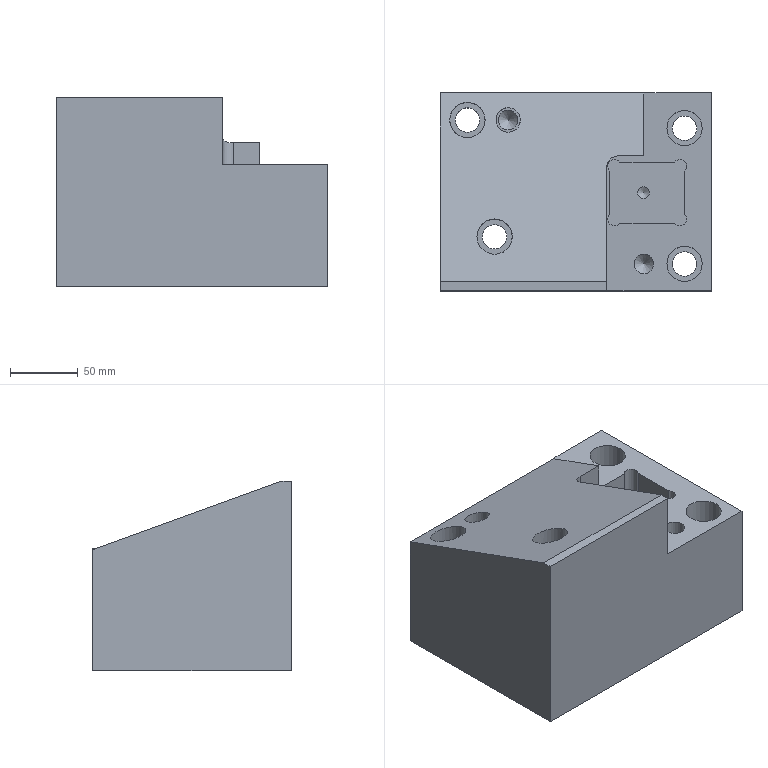Part | STEP file | lll_id5022_x_t | 1 solid | 42 faces | box 200 x 146 x 140 mm | volume 2863405 mm3 | plane 22 | cylinder 17 | cone 3 | commonest cylinder face diameters 10 x4 18.009 x4 26.008 x4 14.506 x2 8.506 x1 16 x1
STEP:
#1=CARTESIAN_POINT('',(2866.996,-53.,0.));
#2=VERTEX_POINT('',#1);
#3=CARTESIAN_POINT('',(2880.,-53.,0.));
#4=DIRECTION('',(0.,0.,1.));
#5=DIRECTION('',(-1.,0.,0.));
#6=AXIS2_PLACEMENT_3D('',#3,#4,#5);
#7=CIRCLE('',#6,13.004);
#8=EDGE_CURVE('',#2,#2,#7,.T.);
#9=ORIENTED_EDGE('',*,*,#8,.F.);
#10=EDGE_LOOP('',(#9));
#11=FACE_BOUND('',#10,.T.);
#12=CARTESIAN_POINT('',(2866.996,-153.,0.));
#13=VERTEX_POINT('',#12);
#14=CARTESIAN_POINT('',(2880.,-153.,0.));
#15=DIRECTION('',(0.,0.,1.));
#16=DIRECTION('',(-1.,0.,0.));
#17=AXIS2_PLACEMENT_3D('',#14,#15,#16);
#18=CIRCLE('',#17,13.004);
#19=EDGE_CURVE('',#13,#13,#18,.T.);
#20=ORIENTED_EDGE('',*,*,#19,.F.);
#21=EDGE_LOOP('',(#20));
#22=FACE_BOUND('',#21,.T.);
#23=CARTESIAN_POINT('',(2822.75,-173.,0.));
#24=VERTEX_POINT('',#23);
#25=CARTESIAN_POINT('',(2822.75,-81.5,0.));
#26=VERTEX_POINT('',#25);
#27=CARTESIAN_POINT('',(2822.75,-150.5,0.));
#28=DIRECTION('',(0.,1.,0.));
#29=VECTOR('',#28,1.);
#30=LINE('',#27,#29);
#31=EDGE_CURVE('',#24,#26,#30,.T.);
#32=ORIENTED_EDGE('',*,*,#31,.F.);
#33=CARTESIAN_POINT('',(2900.,-173.,0.));
#34=VERTEX_POINT('',#33);
#35=CARTESIAN_POINT('',(2692.5,-173.,0.));
#36=DIRECTION('',(-1.,0.,0.));
#37=VECTOR('',#36,1.);
#38=LINE('',#35,#37);
#39=EDGE_CURVE('',#34,#24,#38,.T.);
#40=ORIENTED_EDGE('',*,*,#39,.F.);
#41=CARTESIAN_POINT('',(2900.,-27.,0.));
#42=VERTEX_POINT('',#41);
#43=CARTESIAN_POINT('',(2900.,0.00007613,0.));
#44=DIRECTION('',(0.,1.,0.));
#45=VECTOR('',#44,1.);
#46=LINE('',#43,#45);
#47=EDGE_CURVE('',#34,#42,#46,.T.);
#48=ORIENTED_EDGE('',*,*,#47,.T.);
#49=CARTESIAN_POINT('',(2850.,-27.,0.));
#50=VERTEX_POINT('',#49);
#51=CARTESIAN_POINT('',(2520.,-27.,0.));
#52=DIRECTION('',(1.,0.,0.));
#53=VECTOR('',#52,1.);
#54=LINE('',#51,#53);
#55=EDGE_CURVE('',#50,#42,#54,.T.);
#56=ORIENTED_EDGE('',*,*,#55,.F.);
#57=CARTESIAN_POINT('',(2850.,-28.941,0.));
#58=VERTEX_POINT('',#57);
#59=CARTESIAN_POINT('',(2850.,-102.5,0.));
#60=DIRECTION('',(0.,1.,0.));
#61=VECTOR('',#60,1.);
#62=LINE('',#59,#61);
#63=EDGE_CURVE('',#58,#50,#62,.T.);
#64=ORIENTED_EDGE('',*,*,#63,.F.);
#65=CARTESIAN_POINT('',(2850.,-73.5,0.));
#66=VERTEX_POINT('',#65);
#67=CARTESIAN_POINT('',(2850.,-97.5,0.));
#68=DIRECTION('',(0.,-1.,0.));
#69=VECTOR('',#68,1.);
#70=LINE('',#67,#69);
#71=EDGE_CURVE('',#58,#66,#70,.T.);
#72=ORIENTED_EDGE('',*,*,#71,.T.);
#73=CARTESIAN_POINT('',(2830.75,-73.5,0.));
#74=VERTEX_POINT('',#73);
#75=CARTESIAN_POINT('',(2839.75,-73.5,0.));
#76=DIRECTION('',(1.,0.,0.));
#77=VECTOR('',#76,1.);
#78=LINE('',#75,#77);
#79=EDGE_CURVE('',#74,#66,#78,.T.);
#80=ORIENTED_EDGE('',*,*,#79,.F.);
#81=CARTESIAN_POINT('',(2830.75,-81.5,0.));
#82=DIRECTION('',(0.,0.,-1.));
#83=DIRECTION('',(-1.,0.,0.));
#84=AXIS2_PLACEMENT_3D('',#81,#82,#83);
#85=CIRCLE('',#84,8.);
#86=EDGE_CURVE('',#26,#74,#85,.T.);
#87=ORIENTED_EDGE('',*,*,#86,.F.);
#88=EDGE_LOOP('',(#32,#40,#48,#56,#64,#72,#80,#87));
#89=FACE_BOUND('',#88,.T.);
#90=CARTESIAN_POINT('',(2879.963,-116.273,0.));
#91=VERTEX_POINT('',#90);
#92=CARTESIAN_POINT('',(2879.963,-84.727,0.));
#93=VERTEX_POINT('',#92);
#94=CARTESIAN_POINT('',(2879.963,0.00007613,0.));
#95=DIRECTION('',(0.,1.,0.));
#96=VECTOR('',#95,1.);
#97=LINE('',#94,#96);
#98=EDGE_CURVE('',#91,#93,#97,.T.);
#99=ORIENTED_EDGE('',*,*,#98,.F.);
#100=CARTESIAN_POINT('',(2872.626,-123.,0.));
#101=VERTEX_POINT('',#100);
#102=CARTESIAN_POINT('',(2876.618,-119.989,0.));
#103=DIRECTION('',(0.,0.,1.));
#104=DIRECTION('',(-1.,0.,0.));
#105=AXIS2_PLACEMENT_3D('',#102,#103,#104);
#106=CIRCLE('',#105,5.);
#107=EDGE_CURVE('',#101,#91,#106,.T.);
#108=ORIENTED_EDGE('',*,*,#107,.F.);
#109=CARTESIAN_POINT('',(2832.3,-123.,0.));
#110=VERTEX_POINT('',#109);
#111=CARTESIAN_POINT('',(2772.5,-123.,0.));
#112=DIRECTION('',(1.,0.,0.));
#113=VECTOR('',#112,1.);
#114=LINE('',#111,#113);
#115=EDGE_CURVE('',#110,#101,#114,.T.);
#116=ORIENTED_EDGE('',*,*,#115,.F.);
#117=CARTESIAN_POINT('',(2824.963,-116.273,0.));
#118=VERTEX_POINT('',#117);
#119=CARTESIAN_POINT('',(2828.308,-119.989,0.));
#120=DIRECTION('',(0.,0.,1.));
#121=DIRECTION('',(-1.,0.,0.));
#122=AXIS2_PLACEMENT_3D('',#119,#120,#121);
#123=CIRCLE('',#122,5.);
#124=EDGE_CURVE('',#118,#110,#123,.T.);
#125=ORIENTED_EDGE('',*,*,#124,.F.);
#126=CARTESIAN_POINT('',(2824.963,-84.727,0.));
#127=VERTEX_POINT('',#126);
#128=CARTESIAN_POINT('',(2824.963,0.00007613,0.));
#129=DIRECTION('',(0.,-1.,0.));
#130=VECTOR('',#129,1.);
#131=LINE('',#128,#130);
#132=EDGE_CURVE('',#127,#118,#131,.T.);
#133=ORIENTED_EDGE('',*,*,#132,.F.);
#134=CARTESIAN_POINT('',(2832.3,-78.,0.));
#135=VERTEX_POINT('',#134);
#136=CARTESIAN_POINT('',(2828.308,-81.01,0.));
#137=DIRECTION('',(0.,0.,1.));
#138=DIRECTION('',(-1.,0.,0.));
#139=AXIS2_PLACEMENT_3D('',#136,#137,#138);
#140=CIRCLE('',#139,5.);
#141=EDGE_CURVE('',#135,#127,#140,.T.);
#142=ORIENTED_EDGE('',*,*,#141,.F.);
#143=CARTESIAN_POINT('',(2872.626,-78.,0.));
#144=VERTEX_POINT('',#143);
#145=CARTESIAN_POINT('',(2772.5,-78.,0.));
#146=DIRECTION('',(-1.,0.,0.));
#147=VECTOR('',#146,1.);
#148=LINE('',#145,#147);
#149=EDGE_CURVE('',#144,#135,#148,.T.);
#150=ORIENTED_EDGE('',*,*,#149,.F.);
#151=CARTESIAN_POINT('',(2876.618,-81.01,0.));
#152=DIRECTION('',(0.,0.,1.));
#153=DIRECTION('',(-1.,0.,0.));
#154=AXIS2_PLACEMENT_3D('',#151,#152,#153);
#155=CIRCLE('',#154,5.);
#156=EDGE_CURVE('',#93,#144,#155,.T.);
#157=ORIENTED_EDGE('',*,*,#156,.F.);
#158=EDGE_LOOP('',(#99,#108,#116,#125,#133,#142,#150,#157));
#159=FACE_BOUND('',#158,.T.);
#160=CARTESIAN_POINT('',(2842.747,-153.,0.));
#161=VERTEX_POINT('',#160);
#162=CARTESIAN_POINT('',(2850.,-153.,0.));
#163=DIRECTION('',(0.,0.,-1.));
#164=DIRECTION('',(-1.,0.,0.));
#165=AXIS2_PLACEMENT_3D('',#162,#163,#164);
#166=CIRCLE('',#165,7.253);
#167=EDGE_CURVE('',#161,#161,#166,.T.);
#168=ORIENTED_EDGE('',*,*,#167,.T.);
#169=EDGE_LOOP('',(#168));
#170=FACE_BOUND('',#169,.T.);
#171=CARTESIAN_POINT('',(2772.5,0.00007613,0.));
#172=DIRECTION('',(0.,0.,1.));
#173=DIRECTION('',(1.,0.,0.));
#174=AXIS2_PLACEMENT_3D('',#171,#172,#173);
#175=PLANE('',#174);
#176=ADVANCED_FACE('',(#11,#22,#89,#159,#170),#175,.T.);
#177=CARTESIAN_POINT('',(2822.75,-173.,50.));
#178=VERTEX_POINT('',#177);
#179=CARTESIAN_POINT('',(2700.,-173.,50.));
#180=VERTEX_POINT('',#179);
#181=CARTESIAN_POINT('',(2692.5,-173.,50.));
#182=DIRECTION('',(-1.,0.,0.));
#183=VECTOR('',#182,1.);
#184=LINE('',#181,#183);
#185=EDGE_CURVE('',#178,#180,#184,.T.);
#186=ORIENTED_EDGE('',*,*,#185,.T.);
#187=CARTESIAN_POINT('',(2700.,-173.,-90.));
#188=VERTEX_POINT('',#187);
#189=CARTESIAN_POINT('',(2700.,-173.,6.));
#190=DIRECTION('',(0.,0.,-1.));
#191=VECTOR('',#190,1.);
#192=LINE('',#189,#191);
#193=EDGE_CURVE('',#180,#188,#192,.T.);
#194=ORIENTED_EDGE('',*,*,#193,.T.);
#195=CARTESIAN_POINT('',(2900.,-173.,-90.));
#196=VERTEX_POINT('',#195);
#197=CARTESIAN_POINT('',(-2196.249,-173.,-90.));
#198=DIRECTION('',(1.,0.,0.));
#199=VECTOR('',#198,1.);
#200=LINE('',#197,#199);
#201=EDGE_CURVE('',#188,#196,#200,.T.);
#202=ORIENTED_EDGE('',*,*,#201,.T.);
#203=CARTESIAN_POINT('',(2900.,-173.,-80.));
#204=DIRECTION('',(0.,0.,1.));
#205=VECTOR('',#204,1.);
#206=LINE('',#203,#205);
#207=EDGE_CURVE('',#196,#34,#206,.T.);
#208=ORIENTED_EDGE('',*,*,#207,.T.);
#209=ORIENTED_EDGE('',*,*,#39,.T.);
#210=CARTESIAN_POINT('',(2822.75,-173.,6.));
#211=DIRECTION('',(0.,0.,1.));
#212=VECTOR('',#211,1.);
#213=LINE('',#210,#212);
#214=EDGE_CURVE('',#24,#178,#213,.T.);
#215=ORIENTED_EDGE('',*,*,#214,.T.);
#216=EDGE_LOOP('',(#186,#194,#202,#208,#209,#215));
#217=FACE_OUTER_BOUND('',#216,.T.);
#218=CARTESIAN_POINT('',(2692.5,-173.,6.));
#219=DIRECTION('',(0.,-1.,0.));
#220=DIRECTION('',(0.,0.,-1.));
#221=AXIS2_PLACEMENT_3D('',#218,#219,#220);
#222=PLANE('',#221);
#223=ADVANCED_FACE('',(#217),#222,.T.);
#224=CARTESIAN_POINT('',(2700.,-27.,-90.));
#225=VERTEX_POINT('',#224);
#226=CARTESIAN_POINT('',(2700.,-27.,-0.7065));
#227=VERTEX_POINT('',#226);
#228=CARTESIAN_POINT('',(2700.,-27.,-80.));
#229=DIRECTION('',(0.,0.,1.));
#230=VECTOR('',#229,1.);
#231=LINE('',#228,#230);
#232=EDGE_CURVE('',#225,#227,#231,.T.);
#233=ORIENTED_EDGE('',*,*,#232,.T.);
#234=CARTESIAN_POINT('',(2850.,-27.,-0.7065));
#235=VERTEX_POINT('',#234);
#236=CARTESIAN_POINT('',(2872.426,-27.,-0.7065));
#237=DIRECTION('',(1.,0.,0.));
#238=VECTOR('',#237,1.);
#239=LINE('',#236,#238);
#240=EDGE_CURVE('',#227,#235,#239,.T.);
#241=ORIENTED_EDGE('',*,*,#240,.T.);
#242=CARTESIAN_POINT('',(2850.,-27.,-80.));
#243=DIRECTION('',(0.,0.,1.));
#244=VECTOR('',#243,1.);
#245=LINE('',#242,#244);
#246=EDGE_CURVE('',#235,#50,#245,.T.);
#247=ORIENTED_EDGE('',*,*,#246,.T.);
#248=ORIENTED_EDGE('',*,*,#55,.T.);
#249=CARTESIAN_POINT('',(2900.,-27.,-90.));
#250=VERTEX_POINT('',#249);
#251=CARTESIAN_POINT('',(2900.,-27.,-80.));
#252=DIRECTION('',(0.,0.,1.));
#253=VECTOR('',#252,1.);
#254=LINE('',#251,#253);
#255=EDGE_CURVE('',#250,#42,#254,.T.);
#256=ORIENTED_EDGE('',*,*,#255,.F.);
#257=CARTESIAN_POINT('',(-2196.249,-27.,-90.));
#258=DIRECTION('',(1.,0.,0.));
#259=VECTOR('',#258,1.);
#260=LINE('',#257,#259);
#261=EDGE_CURVE('',#225,#250,#260,.T.);
#262=ORIENTED_EDGE('',*,*,#261,.F.);
#263=EDGE_LOOP('',(#233,#241,#247,#248,#256,#262));
#264=FACE_OUTER_BOUND('',#263,.T.);
#265=CARTESIAN_POINT('',(2520.,-27.,-80.));
#266=DIRECTION('',(0.,-1.,0.));
#267=DIRECTION('',(0.,0.,1.));
#268=AXIS2_PLACEMENT_3D('',#265,#266,#267);
#269=PLANE('',#268);
#270=ADVANCED_FACE('',(#264),#269,.F.);
#271=CARTESIAN_POINT('',(2740.,-119.996,33.141));
#272=VERTEX_POINT('',#271);
#273=CARTESIAN_POINT('',(2740.,-133.,37.874));
#274=DIRECTION('',(0.,-0.342,-0.9397));
#275=DIRECTION('',(0.,0.9397,-0.342));
#276=AXIS2_PLACEMENT_3D('',#273,#274,#275);
#277=ELLIPSE('',#276,13.839,13.004);
#278=EDGE_CURVE('',#272,#272,#277,.T.);
#279=ORIENTED_EDGE('',*,*,#278,.T.);
#280=EDGE_LOOP('',(#279));
#281=FACE_BOUND('',#280,.T.);
#282=CARTESIAN_POINT('',(2720.,-33.996,1.84));
#283=VERTEX_POINT('',#282);
#284=CARTESIAN_POINT('',(2720.,-47.,6.573));
#285=DIRECTION('',(0.,-0.342,-0.9397));
#286=DIRECTION('',(0.,0.9397,-0.342));
#287=AXIS2_PLACEMENT_3D('',#284,#285,#286);
#288=ELLIPSE('',#287,13.839,13.004);
#289=EDGE_CURVE('',#283,#283,#288,.T.);
#290=ORIENTED_EDGE('',*,*,#289,.T.);
#291=EDGE_LOOP('',(#290));
#292=FACE_BOUND('',#291,.T.);
#293=CARTESIAN_POINT('',(2750.,-38.,3.297));
#294=VERTEX_POINT('',#293);
#295=CARTESIAN_POINT('',(2750.,-47.,6.573));
#296=DIRECTION('',(0.,-0.342,-0.9397));
#297=DIRECTION('',(0.,0.9397,-0.342));
#298=AXIS2_PLACEMENT_3D('',#295,#296,#297);
#299=ELLIPSE('',#298,9.578,9.);
#300=EDGE_CURVE('',#294,#294,#299,.T.);
#301=ORIENTED_EDGE('',*,*,#300,.T.);
#302=EDGE_LOOP('',(#301));
#303=FACE_BOUND('',#302,.T.);
#304=CARTESIAN_POINT('',(2700.,-166.315,50.));
#305=VERTEX_POINT('',#304);
#306=CARTESIAN_POINT('',(2822.75,-166.315,50.));
#307=VERTEX_POINT('',#306);
#308=CARTESIAN_POINT('',(2872.426,-166.315,50.));
#309=DIRECTION('',(1.,0.,0.));
#310=VECTOR('',#309,1.);
#311=LINE('',#308,#310);
#312=EDGE_CURVE('',#305,#307,#311,.T.);
#313=ORIENTED_EDGE('',*,*,#312,.T.);
#314=CARTESIAN_POINT('',(2822.75,-81.5,19.13));
#315=VERTEX_POINT('',#314);
#316=CARTESIAN_POINT('',(2822.75,-20.898,-2.927));
#317=DIRECTION('',(0.,0.9397,-0.342));
#318=VECTOR('',#317,1.);
#319=LINE('',#316,#318);
#320=EDGE_CURVE('',#307,#315,#319,.T.);
#321=ORIENTED_EDGE('',*,*,#320,.T.);
#322=CARTESIAN_POINT('',(2830.75,-73.5,16.218));
#323=VERTEX_POINT('',#322);
#324=CARTESIAN_POINT('',(2830.75,-81.5,19.13));
#325=DIRECTION('',(0.,0.342,0.9397));
#326=DIRECTION('',(0.,-0.9397,0.342));
#327=AXIS2_PLACEMENT_3D('',#324,#325,#326);
#328=ELLIPSE('',#327,8.513,8.);
#329=EDGE_CURVE('',#323,#315,#328,.T.);
#330=ORIENTED_EDGE('',*,*,#329,.F.);
#331=CARTESIAN_POINT('',(2850.,-73.5,16.218));
#332=VERTEX_POINT('',#331);
#333=CARTESIAN_POINT('',(2872.426,-73.5,16.218));
#334=DIRECTION('',(1.,0.,0.));
#335=VECTOR('',#334,1.);
#336=LINE('',#333,#335);
#337=EDGE_CURVE('',#323,#332,#336,.T.);
#338=ORIENTED_EDGE('',*,*,#337,.T.);
#339=CARTESIAN_POINT('',(2850.,-20.898,-2.927));
#340=DIRECTION('',(0.,-0.9397,0.342));
#341=VECTOR('',#340,1.);
#342=LINE('',#339,#341);
#343=EDGE_CURVE('',#58,#332,#342,.T.);
#344=ORIENTED_EDGE('',*,*,#343,.F.);
#345=CARTESIAN_POINT('',(2850.,-85.693,20.656));
#346=DIRECTION('',(0.,-0.9397,0.342));
#347=VECTOR('',#346,1.);
#348=LINE('',#345,#347);
#349=EDGE_CURVE('',#235,#58,#348,.T.);
#350=ORIENTED_EDGE('',*,*,#349,.F.);
#351=ORIENTED_EDGE('',*,*,#240,.F.);
#352=CARTESIAN_POINT('',(2700.,-20.898,-2.927));
#353=DIRECTION('',(0.,0.9397,-0.342));
#354=VECTOR('',#353,1.);
#355=LINE('',#352,#354);
#356=EDGE_CURVE('',#305,#227,#355,.T.);
#357=ORIENTED_EDGE('',*,*,#356,.F.);
#358=EDGE_LOOP('',(#313,#321,#330,#338,#344,#350,#351,#357));
#359=FACE_BOUND('',#358,.T.);
#360=CARTESIAN_POINT('',(2872.426,-20.898,-2.927));
#361=DIRECTION('',(0.,0.342,0.9397));
#362=DIRECTION('',(0.,-0.9397,0.342));
#363=AXIS2_PLACEMENT_3D('',#360,#361,#362);
#364=PLANE('',#363);
#365=ADVANCED_FACE('',(#281,#292,#303,#359),#364,.T.);
#366=CARTESIAN_POINT('',(2749.004,-133.,-90.));
#367=VERTEX_POINT('',#366);
#368=CARTESIAN_POINT('',(2740.,-133.,-90.));
#369=DIRECTION('',(0.,0.,1.));
#370=DIRECTION('',(1.,0.,0.));
#371=AXIS2_PLACEMENT_3D('',#368,#369,#370);
#372=CIRCLE('',#371,9.005);
#373=EDGE_CURVE('',#367,#367,#372,.T.);
#374=ORIENTED_EDGE('',*,*,#373,.T.);
#375=EDGE_LOOP('',(#374));
#376=FACE_BOUND('',#375,.T.);
#377=CARTESIAN_POINT('',(2729.004,-47.,-90.));
#378=VERTEX_POINT('',#377);
#379=CARTESIAN_POINT('',(2720.,-47.,-90.));
#380=DIRECTION('',(0.,0.,1.));
#381=DIRECTION('',(1.,0.,0.));
#382=AXIS2_PLACEMENT_3D('',#379,#380,#381);
#383=CIRCLE('',#382,9.005);
#384=EDGE_CURVE('',#378,#378,#383,.T.);
#385=ORIENTED_EDGE('',*,*,#384,.T.);
#386=EDGE_LOOP('',(#385));
#387=FACE_BOUND('',#386,.T.);
#388=CARTESIAN_POINT('',(2889.005,-53.,-90.));
#389=VERTEX_POINT('',#388);
#390=CARTESIAN_POINT('',(2880.,-53.,-90.));
#391=DIRECTION('',(0.,0.,1.));
#392=DIRECTION('',(1.,0.,0.));
#393=AXIS2_PLACEMENT_3D('',#390,#391,#392);
#394=CIRCLE('',#393,9.005);
#395=EDGE_CURVE('',#389,#389,#394,.T.);
#396=ORIENTED_EDGE('',*,*,#395,.T.);
#397=EDGE_LOOP('',(#396));
#398=FACE_BOUND('',#397,.T.);
#399=CARTESIAN_POINT('',(2889.005,-153.,-90.));
#400=VERTEX_POINT('',#399);
#401=CARTESIAN_POINT('',(2880.,-153.,-90.));
#402=DIRECTION('',(0.,0.,1.));
#403=DIRECTION('',(1.,0.,0.));
#404=AXIS2_PLACEMENT_3D('',#401,#402,#403);
#405=CIRCLE('',#404,9.005);
#406=EDGE_CURVE('',#400,#400,#405,.T.);
#407=ORIENTED_EDGE('',*,*,#406,.T.);
#408=EDGE_LOOP('',(#407));
#409=FACE_BOUND('',#408,.T.);
#410=ORIENTED_EDGE('',*,*,#261,.T.);
#411=CARTESIAN_POINT('',(2900.,1.,-90.));
#412=DIRECTION('',(0.,1.,0.));
#413=VECTOR('',#412,1.);
#414=LINE('',#411,#413);
#415=EDGE_CURVE('',#196,#250,#414,.T.);
#416=ORIENTED_EDGE('',*,*,#415,.F.);
#417=ORIENTED_EDGE('',*,*,#201,.F.);
#418=CARTESIAN_POINT('',(2700.,-97.5,-90.));
#419=DIRECTION('',(0.,1.,0.));
#420=VECTOR('',#419,1.);
#421=LINE('',#418,#420);
#422=EDGE_CURVE('',#188,#225,#421,.T.);
#423=ORIENTED_EDGE('',*,*,#422,.T.);
#424=EDGE_LOOP('',(#410,#416,#417,#423));
#425=FACE_BOUND('',#424,.T.);
#426=CARTESIAN_POINT('',(-2196.249,1.,-90.));
#427=DIRECTION('',(0.,0.,-1.));
#428=DIRECTION('',(1.,0.,0.));
#429=AXIS2_PLACEMENT_3D('',#426,#427,#428);
#430=PLANE('',#429);
#431=ADVANCED_FACE('',(#376,#387,#398,#409,#425),#430,.T.);
#432=ORIENTED_EDGE('',*,*,#79,.T.);
#433=CARTESIAN_POINT('',(2850.,-73.5,0.));
#434=DIRECTION('',(0.,0.,1.));
#435=VECTOR('',#434,1.);
#436=LINE('',#433,#435);
#437=EDGE_CURVE('',#66,#332,#436,.T.);
#438=ORIENTED_EDGE('',*,*,#437,.T.);
#439=ORIENTED_EDGE('',*,*,#337,.F.);
#440=CARTESIAN_POINT('',(2830.75,-73.5,16.218));
#441=DIRECTION('',(0.,0.,1.));
#442=VECTOR('',#441,1.);
#443=LINE('',#440,#442);
#444=EDGE_CURVE('',#74,#323,#443,.T.);
#445=ORIENTED_EDGE('',*,*,#444,.F.);
#446=EDGE_LOOP('',(#432,#438,#439,#445));
#447=FACE_OUTER_BOUND('',#446,.T.);
#448=CARTESIAN_POINT('',(2839.75,-73.5,0.));
#449=DIRECTION('',(0.,1.,0.));
#450=DIRECTION('',(0.,0.,1.));
#451=AXIS2_PLACEMENT_3D('',#448,#449,#450);
#452=PLANE('',#451);
#453=ADVANCED_FACE('',(#447),#452,.F.);
#454=ORIENTED_EDGE('',*,*,#214,.F.);
#455=ORIENTED_EDGE('',*,*,#31,.T.);
#456=CARTESIAN_POINT('',(2822.75,-81.5,0.));
#457=DIRECTION('',(0.,0.,-1.));
#458=VECTOR('',#457,1.);
#459=LINE('',#456,#458);
#460=EDGE_CURVE('',#315,#26,#459,.T.);
#461=ORIENTED_EDGE('',*,*,#460,.F.);
#462=ORIENTED_EDGE('',*,*,#320,.F.);
#463=CARTESIAN_POINT('',(2822.75,97.5,50.));
#464=DIRECTION('',(0.,-1.,0.));
#465=VECTOR('',#464,1.);
#466=LINE('',#463,#465);
#467=EDGE_CURVE('',#307,#178,#466,.T.);
#468=ORIENTED_EDGE('',*,*,#467,.T.);
#469=EDGE_LOOP('',(#454,#455,#461,#462,#468));
#470=FACE_OUTER_BOUND('',#469,.T.);
#471=CARTESIAN_POINT('',(2822.75,-150.5,0.));
#472=DIRECTION('',(-1.,0.,0.));
#473=DIRECTION('',(0.,0.,-1.));
#474=AXIS2_PLACEMENT_3D('',#471,#472,#473);
#475=PLANE('',#474);
#476=ADVANCED_FACE('',(#470),#475,.F.);
#477=ORIENTED_EDGE('',*,*,#71,.F.);
#478=ORIENTED_EDGE('',*,*,#343,.T.);
#479=ORIENTED_EDGE('',*,*,#437,.F.);
#480=EDGE_LOOP('',(#477,#478,#479));
#481=FACE_OUTER_BOUND('',#480,.T.);
#482=CARTESIAN_POINT('',(2850.,-97.5,-25.521));
#483=DIRECTION('',(1.,0.,0.));
#484=DIRECTION('',(0.,0.,1.));
#485=AXIS2_PLACEMENT_3D('',#482,#483,#484);
#486=PLANE('',#485);
#487=ADVANCED_FACE('',(#481),#486,.T.);
#488=ORIENTED_EDGE('',*,*,#415,.T.);
#489=ORIENTED_EDGE('',*,*,#255,.T.);
#490=ORIENTED_EDGE('',*,*,#47,.F.);
#491=ORIENTED_EDGE('',*,*,#207,.F.);
#492=EDGE_LOOP('',(#488,#489,#490,#491));
#493=FACE_OUTER_BOUND('',#492,.T.);
#494=CARTESIAN_POINT('',(2900.,-335.,-80.));
#495=DIRECTION('',(1.,0.,0.));
#496=DIRECTION('',(0.,0.,1.));
#497=AXIS2_PLACEMENT_3D('',#494,#495,#496);
#498=PLANE('',#497);
#499=ADVANCED_FACE('',(#493),#498,.T.);
#500=ORIENTED_EDGE('',*,*,#349,.T.);
#501=ORIENTED_EDGE('',*,*,#63,.T.);
#502=ORIENTED_EDGE('',*,*,#246,.F.);
#503=EDGE_LOOP('',(#500,#501,#502));
#504=FACE_OUTER_BOUND('',#503,.T.);
#505=CARTESIAN_POINT('',(2850.,-102.5,-25.521));
#506=DIRECTION('',(1.,0.,0.));
#507=DIRECTION('',(0.,0.,1.));
#508=AXIS2_PLACEMENT_3D('',#505,#506,#507);
#509=PLANE('',#508);
#510=ADVANCED_FACE('',(#504),#509,.F.);
#511=ORIENTED_EDGE('',*,*,#329,.T.);
#512=ORIENTED_EDGE('',*,*,#460,.T.);
#513=ORIENTED_EDGE('',*,*,#86,.T.);
#514=ORIENTED_EDGE('',*,*,#444,.T.);
#515=EDGE_LOOP('',(#511,#512,#513,#514));
#516=FACE_OUTER_BOUND('',#515,.T.);
#517=CARTESIAN_POINT('',(2830.75,-81.5,0.));
#518=DIRECTION('',(0.,0.,1.));
#519=DIRECTION('',(-1.,0.,0.));
#520=AXIS2_PLACEMENT_3D('',#517,#518,#519);
#521=CYLINDRICAL_SURFACE('',#520,8.);
#522=ADVANCED_FACE('',(#516),#521,.F.);
#523=CARTESIAN_POINT('',(2700.,97.5,50.));
#524=DIRECTION('',(0.,-1.,0.));
#525=VECTOR('',#524,1.);
#526=LINE('',#523,#525);
#527=EDGE_CURVE('',#305,#180,#526,.T.);
#528=ORIENTED_EDGE('',*,*,#527,.F.);
#529=ORIENTED_EDGE('',*,*,#356,.T.);
#530=ORIENTED_EDGE('',*,*,#232,.F.);
#531=ORIENTED_EDGE('',*,*,#422,.F.);
#532=ORIENTED_EDGE('',*,*,#193,.F.);
#533=EDGE_LOOP('',(#528,#529,#530,#531,#532));
#534=FACE_OUTER_BOUND('',#533,.T.);
#535=CARTESIAN_POINT('',(2700.,-97.5,-7.593));
#536=DIRECTION('',(-1.,0.,0.));
#537=DIRECTION('',(0.,0.,-1.));
#538=AXIS2_PLACEMENT_3D('',#535,#536,#537);
#539=PLANE('',#538);
#540=ADVANCED_FACE('',(#534),#539,.T.);
#541=CARTESIAN_POINT('',(2832.3,-123.,-20.));
#542=VERTEX_POINT('',#541);
#543=CARTESIAN_POINT('',(2832.3,-123.,-20.));
#544=DIRECTION('',(0.,0.,1.));
#545=VECTOR('',#544,1.);
#546=LINE('',#543,#545);
#547=EDGE_CURVE('',#542,#110,#546,.T.);
#548=ORIENTED_EDGE('',*,*,#547,.T.);
#549=ORIENTED_EDGE('',*,*,#115,.T.);
#550=CARTESIAN_POINT('',(2872.626,-123.,-20.));
#551=VERTEX_POINT('',#550);
#552=CARTESIAN_POINT('',(2872.626,-123.,-20.));
#553=DIRECTION('',(0.,0.,-1.));
#554=VECTOR('',#553,1.);
#555=LINE('',#552,#554);
#556=EDGE_CURVE('',#101,#551,#555,.T.);
#557=ORIENTED_EDGE('',*,*,#556,.T.);
#558=CARTESIAN_POINT('',(2849.963,-123.,-20.));
#559=DIRECTION('',(1.,0.,0.));
#560=VECTOR('',#559,1.);
#561=LINE('',#558,#560);
#562=EDGE_CURVE('',#542,#551,#561,.T.);
#563=ORIENTED_EDGE('',*,*,#562,.F.);
#564=EDGE_LOOP('',(#548,#549,#557,#563));
#565=FACE_OUTER_BOUND('',#564,.T.);
#566=CARTESIAN_POINT('',(2849.963,-123.,-20.));
#567=DIRECTION('',(0.,-1.,0.));
#568=DIRECTION('',(0.,0.,-1.));
#569=AXIS2_PLACEMENT_3D('',#566,#567,#568);
#570=PLANE('',#569);
#571=ADVANCED_FACE('',(#565),#570,.F.);
#572=CARTESIAN_POINT('',(2879.963,-116.273,-20.));
#573=VERTEX_POINT('',#572);
#574=CARTESIAN_POINT('',(2879.963,-116.273,-20.));
#575=DIRECTION('',(0.,0.,1.));
#576=VECTOR('',#575,1.);
#577=LINE('',#574,#576);
#578=EDGE_CURVE('',#573,#91,#577,.T.);
#579=ORIENTED_EDGE('',*,*,#578,.T.);
#580=ORIENTED_EDGE('',*,*,#98,.T.);
#581=CARTESIAN_POINT('',(2879.963,-84.727,-20.));
#582=VERTEX_POINT('',#581);
#583=CARTESIAN_POINT('',(2879.963,-84.727,-20.));
#584=DIRECTION('',(0.,0.,-1.));
#585=VECTOR('',#584,1.);
#586=LINE('',#583,#585);
#587=EDGE_CURVE('',#93,#582,#586,.T.);
#588=ORIENTED_EDGE('',*,*,#587,.T.);
#589=CARTESIAN_POINT('',(2879.963,-100.5,-20.));
#590=DIRECTION('',(0.,1.,0.));
#591=VECTOR('',#590,1.);
#592=LINE('',#589,#591);
#593=EDGE_CURVE('',#573,#582,#592,.T.);
#594=ORIENTED_EDGE('',*,*,#593,.F.);
#595=EDGE_LOOP('',(#579,#580,#588,#594));
#596=FACE_OUTER_BOUND('',#595,.T.);
#597=CARTESIAN_POINT('',(2879.963,-100.5,-20.));
#598=DIRECTION('',(1.,0.,0.));
#599=DIRECTION('',(0.,0.,1.));
#600=AXIS2_PLACEMENT_3D('',#597,#598,#599);
#601=PLANE('',#600);
#602=ADVANCED_FACE('',(#596),#601,.F.);
#603=CARTESIAN_POINT('',(2872.626,-78.,-20.));
#604=VERTEX_POINT('',#603);
#605=CARTESIAN_POINT('',(2872.626,-78.,-20.));
#606=DIRECTION('',(0.,0.,1.));
#607=VECTOR('',#606,1.);
#608=LINE('',#605,#607);
#609=EDGE_CURVE('',#604,#144,#608,.T.);
#610=ORIENTED_EDGE('',*,*,#609,.T.);
#611=ORIENTED_EDGE('',*,*,#149,.T.);
#612=CARTESIAN_POINT('',(2832.3,-78.,-20.));
#613=VERTEX_POINT('',#612);
#614=CARTESIAN_POINT('',(2832.3,-78.,-20.));
#615=DIRECTION('',(0.,0.,-1.));
#616=VECTOR('',#615,1.);
#617=LINE('',#614,#616);
#618=EDGE_CURVE('',#135,#613,#617,.T.);
#619=ORIENTED_EDGE('',*,*,#618,.T.);
#620=CARTESIAN_POINT('',(2849.963,-78.,-20.));
#621=DIRECTION('',(-1.,0.,0.));
#622=VECTOR('',#621,1.);
#623=LINE('',#620,#622);
#624=EDGE_CURVE('',#604,#613,#623,.T.);
#625=ORIENTED_EDGE('',*,*,#624,.F.);
#626=EDGE_LOOP('',(#610,#611,#619,#625));
#627=FACE_OUTER_BOUND('',#626,.T.);
#628=CARTESIAN_POINT('',(2849.963,-78.,-20.));
#629=DIRECTION('',(0.,1.,0.));
#630=DIRECTION('',(0.,0.,1.));
#631=AXIS2_PLACEMENT_3D('',#628,#629,#630);
#632=PLANE('',#631);
#633=ADVANCED_FACE('',(#627),#632,.F.);
#634=CARTESIAN_POINT('',(2824.963,-84.727,-20.));
#635=VERTEX_POINT('',#634);
#636=CARTESIAN_POINT('',(2824.963,-84.727,-20.));
#637=DIRECTION('',(0.,0.,1.));
#638=VECTOR('',#637,1.);
#639=LINE('',#636,#638);
#640=EDGE_CURVE('',#635,#127,#639,.T.);
#641=ORIENTED_EDGE('',*,*,#640,.T.);
#642=ORIENTED_EDGE('',*,*,#132,.T.);
#643=CARTESIAN_POINT('',(2824.963,-116.273,-20.));
#644=VERTEX_POINT('',#643);
#645=CARTESIAN_POINT('',(2824.963,-116.273,-20.));
#646=DIRECTION('',(0.,0.,-1.));
#647=VECTOR('',#646,1.);
#648=LINE('',#645,#647);
#649=EDGE_CURVE('',#118,#644,#648,.T.);
#650=ORIENTED_EDGE('',*,*,#649,.T.);
#651=CARTESIAN_POINT('',(2824.963,-100.5,-20.));
#652=DIRECTION('',(0.,-1.,0.));
#653=VECTOR('',#652,1.);
#654=LINE('',#651,#653);
#655=EDGE_CURVE('',#635,#644,#654,.T.);
#656=ORIENTED_EDGE('',*,*,#655,.F.);
#657=EDGE_LOOP('',(#641,#642,#650,#656));
#658=FACE_OUTER_BOUND('',#657,.T.);
#659=CARTESIAN_POINT('',(2824.963,-100.5,-20.));
#660=DIRECTION('',(-1.,0.,0.));
#661=DIRECTION('',(0.,0.,-1.));
#662=AXIS2_PLACEMENT_3D('',#659,#660,#661);
#663=PLANE('',#662);
#664=ADVANCED_FACE('',(#658),#663,.F.);
#665=ORIENTED_EDGE('',*,*,#556,.F.);
#666=ORIENTED_EDGE('',*,*,#107,.T.);
#667=ORIENTED_EDGE('',*,*,#578,.F.);
#668=CARTESIAN_POINT('',(2876.618,-119.989,-20.));
#669=DIRECTION('',(0.,0.,1.));
#670=DIRECTION('',(-1.,0.,0.));
#671=AXIS2_PLACEMENT_3D('',#668,#669,#670);
#672=CIRCLE('',#671,5.);
#673=EDGE_CURVE('',#551,#573,#672,.T.);
#674=ORIENTED_EDGE('',*,*,#673,.F.);
#675=EDGE_LOOP('',(#665,#666,#667,#674));
#676=FACE_OUTER_BOUND('',#675,.T.);
#677=CARTESIAN_POINT('',(2876.618,-119.989,-20.));
#678=DIRECTION('',(0.,0.,1.));
#679=DIRECTION('',(-1.,0.,0.));
#680=AXIS2_PLACEMENT_3D('',#677,#678,#679);
#681=CYLINDRICAL_SURFACE('',#680,5.);
#682=ADVANCED_FACE('',(#676),#681,.F.);
#683=ORIENTED_EDGE('',*,*,#618,.F.);
#684=ORIENTED_EDGE('',*,*,#141,.T.);
#685=ORIENTED_EDGE('',*,*,#640,.F.);
#686=CARTESIAN_POINT('',(2828.308,-81.01,-20.));
#687=DIRECTION('',(0.,0.,1.));
#688=DIRECTION('',(-1.,0.,0.));
#689=AXIS2_PLACEMENT_3D('',#686,#687,#688);
#690=CIRCLE('',#689,5.);
#691=EDGE_CURVE('',#613,#635,#690,.T.);
#692=ORIENTED_EDGE('',*,*,#691,.F.);
#693=EDGE_LOOP('',(#683,#684,#685,#692));
#694=FACE_OUTER_BOUND('',#693,.T.);
#695=CARTESIAN_POINT('',(2828.308,-81.01,-20.));
#696=DIRECTION('',(0.,0.,1.));
#697=DIRECTION('',(-1.,0.,0.));
#698=AXIS2_PLACEMENT_3D('',#695,#696,#697);
#699=CYLINDRICAL_SURFACE('',#698,5.);
#700=ADVANCED_FACE('',(#694),#699,.F.);
#701=ORIENTED_EDGE('',*,*,#587,.F.);
#702=ORIENTED_EDGE('',*,*,#156,.T.);
#703=ORIENTED_EDGE('',*,*,#609,.F.);
#704=CARTESIAN_POINT('',(2876.618,-81.01,-20.));
#705=DIRECTION('',(0.,0.,1.));
#706=DIRECTION('',(-1.,0.,0.));
#707=AXIS2_PLACEMENT_3D('',#704,#705,#706);
#708=CIRCLE('',#707,5.);
#709=EDGE_CURVE('',#582,#604,#708,.T.);
#710=ORIENTED_EDGE('',*,*,#709,.F.);
#711=EDGE_LOOP('',(#701,#702,#703,#710));
#712=FACE_OUTER_BOUND('',#711,.T.);
#713=CARTESIAN_POINT('',(2876.618,-81.01,-20.));
#714=DIRECTION('',(0.,0.,1.));
#715=DIRECTION('',(-1.,0.,0.));
#716=AXIS2_PLACEMENT_3D('',#713,#714,#715);
#717=CYLINDRICAL_SURFACE('',#716,5.);
#718=ADVANCED_FACE('',(#712),#717,.F.);
#719=ORIENTED_EDGE('',*,*,#649,.F.);
#720=ORIENTED_EDGE('',*,*,#124,.T.);
#721=ORIENTED_EDGE('',*,*,#547,.F.);
#722=CARTESIAN_POINT('',(2828.308,-119.989,-20.));
#723=DIRECTION('',(0.,0.,1.));
#724=DIRECTION('',(-1.,0.,0.));
#725=AXIS2_PLACEMENT_3D('',#722,#723,#724);
#726=CIRCLE('',#725,5.);
#727=EDGE_CURVE('',#644,#542,#726,.T.);
#728=ORIENTED_EDGE('',*,*,#727,.F.);
#729=EDGE_LOOP('',(#719,#720,#721,#728));
#730=FACE_OUTER_BOUND('',#729,.T.);
#731=CARTESIAN_POINT('',(2828.308,-119.989,-20.));
#732=DIRECTION('',(0.,0.,1.));
#733=DIRECTION('',(-1.,0.,0.));
#734=AXIS2_PLACEMENT_3D('',#731,#732,#733);
#735=CYLINDRICAL_SURFACE('',#734,5.);
#736=ADVANCED_FACE('',(#730),#735,.F.);
#737=CARTESIAN_POINT('',(2845.464,-100.5,-20.));
#738=VERTEX_POINT('',#737);
#739=CARTESIAN_POINT('',(2849.717,-100.5,-20.));
#740=DIRECTION('',(0.,0.,-1.));
#741=DIRECTION('',(-1.,0.,0.));
#742=AXIS2_PLACEMENT_3D('',#739,#740,#741);
#743=CIRCLE('',#742,4.253);
#744=EDGE_CURVE('',#738,#738,#743,.T.);
#745=ORIENTED_EDGE('',*,*,#744,.T.);
#746=EDGE_LOOP('',(#745));
#747=FACE_BOUND('',#746,.T.);
#748=ORIENTED_EDGE('',*,*,#655,.T.);
#749=ORIENTED_EDGE('',*,*,#727,.T.);
#750=ORIENTED_EDGE('',*,*,#562,.T.);
#751=ORIENTED_EDGE('',*,*,#673,.T.);
#752=ORIENTED_EDGE('',*,*,#593,.T.);
#753=ORIENTED_EDGE('',*,*,#709,.T.);
#754=ORIENTED_EDGE('',*,*,#624,.T.);
#755=ORIENTED_EDGE('',*,*,#691,.T.);
#756=EDGE_LOOP('',(#748,#749,#750,#751,#752,#753,#754,#755));
#757=FACE_BOUND('',#756,.T.);
#758=CARTESIAN_POINT('',(2849.963,-100.5,-20.));
#759=DIRECTION('',(0.,0.,-1.));
#760=DIRECTION('',(1.,0.,0.));
#761=AXIS2_PLACEMENT_3D('',#758,#759,#760);
#762=PLANE('',#761);
#763=ADVANCED_FACE('',(#747,#757),#762,.F.);
#764=ORIENTED_EDGE('',*,*,#185,.F.);
#765=ORIENTED_EDGE('',*,*,#467,.F.);
#766=ORIENTED_EDGE('',*,*,#312,.F.);
#767=ORIENTED_EDGE('',*,*,#527,.T.);
#768=EDGE_LOOP('',(#764,#765,#766,#767));
#769=FACE_OUTER_BOUND('',#768,.T.);
#770=CARTESIAN_POINT('',(2800.,97.5,50.));
#771=DIRECTION('',(0.,0.,-1.));
#772=DIRECTION('',(1.,0.,0.));
#773=AXIS2_PLACEMENT_3D('',#770,#771,#772);
#774=PLANE('',#773);
#775=ADVANCED_FACE('',(#769),#774,.F.);
#776=CARTESIAN_POINT('',(2757.253,-47.,-5.));
#777=VERTEX_POINT('',#776);
#778=CARTESIAN_POINT('',(2750.,-47.,-5.));
#779=DIRECTION('',(0.,0.,1.));
#780=DIRECTION('',(1.,0.,0.));
#781=AXIS2_PLACEMENT_3D('',#778,#779,#780);
#782=CIRCLE('',#781,7.253);
#783=EDGE_CURVE('',#777,#777,#782,.T.);
#784=ORIENTED_EDGE('',*,*,#783,.F.);
#785=EDGE_LOOP('',(#784));
#786=FACE_BOUND('',#785,.T.);
#787=CARTESIAN_POINT('',(2759.,-47.,-5.));
#788=VERTEX_POINT('',#787);
#789=CARTESIAN_POINT('',(2750.,-47.,-5.));
#790=DIRECTION('',(0.,0.,1.));
#791=DIRECTION('',(1.,0.,0.));
#792=AXIS2_PLACEMENT_3D('',#789,#790,#791);
#793=CIRCLE('',#792,9.);
#794=EDGE_CURVE('',#788,#788,#793,.T.);
#795=ORIENTED_EDGE('',*,*,#794,.T.);
#796=EDGE_LOOP('',(#795));
#797=FACE_BOUND('',#796,.T.);
#798=CARTESIAN_POINT('',(2750.,-47.,-5.));
#799=DIRECTION('',(0.,0.,-1.));
#800=DIRECTION('',(1.,0.,0.));
#801=AXIS2_PLACEMENT_3D('',#798,#799,#800);
#802=PLANE('',#801);
#803=ADVANCED_FACE('',(#786,#797),#802,.F.);
#804=ORIENTED_EDGE('',*,*,#300,.F.);
#805=EDGE_LOOP('',(#804));
#806=FACE_BOUND('',#805,.T.);
#807=ORIENTED_EDGE('',*,*,#794,.F.);
#808=EDGE_LOOP('',(#807));
#809=FACE_BOUND('',#808,.T.);
#810=CARTESIAN_POINT('',(2750.,-47.,10.));
#811=DIRECTION('',(0.,0.,-1.));
#812=DIRECTION('',(-1.,0.,0.));
#813=AXIS2_PLACEMENT_3D('',#810,#811,#812);
#814=CYLINDRICAL_SURFACE('',#813,9.);
#815=ADVANCED_FACE('',(#806,#809),#814,.F.);
#816=CARTESIAN_POINT('',(2857.253,-153.,-37.753));
#817=VERTEX_POINT('',#816);
#818=CARTESIAN_POINT('',(2850.,-153.,-37.753));
#819=DIRECTION('',(0.,0.,-1.));
#820=DIRECTION('',(1.,0.,0.));
#821=AXIS2_PLACEMENT_3D('',#818,#819,#820);
#822=CIRCLE('',#821,7.253);
#823=EDGE_CURVE('',#817,#817,#822,.T.);
#824=ORIENTED_EDGE('',*,*,#823,.T.);
#825=EDGE_LOOP('',(#824));
#826=FACE_BOUND('',#825,.T.);
#827=ORIENTED_EDGE('',*,*,#167,.F.);
#828=EDGE_LOOP('',(#827));
#829=FACE_BOUND('',#828,.T.);
#830=CARTESIAN_POINT('',(2850.,-153.,0.));
#831=DIRECTION('',(0.,0.,-1.));
#832=DIRECTION('',(-1.,0.,0.));
#833=AXIS2_PLACEMENT_3D('',#830,#831,#832);
#834=CYLINDRICAL_SURFACE('',#833,7.253);
#835=ADVANCED_FACE('',(#826,#829),#834,.F.);
#836=CARTESIAN_POINT('',(2850.,-153.,-45.006));
#837=VERTEX_POINT('',#836);
#838=VERTEX_LOOP('',#837);
#839=FACE_BOUND('',#838,.T.);
#840=ORIENTED_EDGE('',*,*,#823,.F.);
#841=EDGE_LOOP('',(#840));
#842=FACE_BOUND('',#841,.T.);
#843=CARTESIAN_POINT('',(2850.,-153.,-37.753));
#844=DIRECTION('',(0.,0.,1.));
#845=DIRECTION('',(-1.,0.,0.));
#846=AXIS2_PLACEMENT_3D('',#843,#844,#845);
#847=CONICAL_SURFACE('',#846,7.253,45.);
#848=ADVANCED_FACE('',(#839,#842),#847,.F.);
#849=CARTESIAN_POINT('',(2757.253,-47.,-27.753));
#850=VERTEX_POINT('',#849);
#851=CARTESIAN_POINT('',(2750.,-47.,-27.753));
#852=DIRECTION('',(0.,0.,-1.));
#853=DIRECTION('',(1.,0.,0.));
#854=AXIS2_PLACEMENT_3D('',#851,#852,#853);
#855=CIRCLE('',#854,7.253);
#856=EDGE_CURVE('',#850,#850,#855,.T.);
#857=ORIENTED_EDGE('',*,*,#856,.T.);
#858=EDGE_LOOP('',(#857));
#859=FACE_BOUND('',#858,.T.);
#860=ORIENTED_EDGE('',*,*,#783,.T.);
#861=EDGE_LOOP('',(#860));
#862=FACE_BOUND('',#861,.T.);
#863=CARTESIAN_POINT('',(2750.,-47.,10.));
#864=DIRECTION('',(0.,0.,-1.));
#865=DIRECTION('',(-1.,0.,0.));
#866=AXIS2_PLACEMENT_3D('',#863,#864,#865);
#867=CYLINDRICAL_SURFACE('',#866,7.253);
#868=ADVANCED_FACE('',(#859,#862),#867,.F.);
#869=CARTESIAN_POINT('',(2750.,-47.,-35.006));
#870=VERTEX_POINT('',#869);
#871=VERTEX_LOOP('',#870);
#872=FACE_BOUND('',#871,.T.);
#873=ORIENTED_EDGE('',*,*,#856,.F.);
#874=EDGE_LOOP('',(#873));
#875=FACE_BOUND('',#874,.T.);
#876=CARTESIAN_POINT('',(2750.,-47.,-27.753));
#877=DIRECTION('',(0.,0.,1.));
#878=DIRECTION('',(-1.,0.,0.));
#879=AXIS2_PLACEMENT_3D('',#876,#877,#878);
#880=CONICAL_SURFACE('',#879,7.253,45.);
#881=ADVANCED_FACE('',(#872,#875),#880,.F.);
#882=CARTESIAN_POINT('',(2866.996,-153.,-50.));
#883=VERTEX_POINT('',#882);
#884=CARTESIAN_POINT('',(2880.,-153.,-50.));
#885=DIRECTION('',(0.,0.,1.));
#886=DIRECTION('',(-1.,0.,0.));
#887=AXIS2_PLACEMENT_3D('',#884,#885,#886);
#888=CIRCLE('',#887,13.004);
#889=EDGE_CURVE('',#883,#883,#888,.T.);
#890=ORIENTED_EDGE('',*,*,#889,.F.);
#891=EDGE_LOOP('',(#890));
#892=FACE_BOUND('',#891,.T.);
#893=ORIENTED_EDGE('',*,*,#19,.T.);
#894=EDGE_LOOP('',(#893));
#895=FACE_BOUND('',#894,.T.);
#896=CARTESIAN_POINT('',(2880.,-153.,50.));
#897=DIRECTION('',(0.,0.,-1.));
#898=DIRECTION('',(-1.,0.,0.));
#899=AXIS2_PLACEMENT_3D('',#896,#897,#898);
#900=CYLINDRICAL_SURFACE('',#899,13.004);
#901=ADVANCED_FACE('',(#892,#895),#900,.F.);
#902=ORIENTED_EDGE('',*,*,#406,.F.);
#903=EDGE_LOOP('',(#902));
#904=FACE_BOUND('',#903,.T.);
#905=CARTESIAN_POINT('',(2889.005,-153.,-50.));
#906=VERTEX_POINT('',#905);
#907=CARTESIAN_POINT('',(2880.,-153.,-50.));
#908=DIRECTION('',(0.,0.,1.));
#909=DIRECTION('',(1.,0.,0.));
#910=AXIS2_PLACEMENT_3D('',#907,#908,#909);
#911=CIRCLE('',#910,9.005);
#912=EDGE_CURVE('',#906,#906,#911,.T.);
#913=ORIENTED_EDGE('',*,*,#912,.T.);
#914=EDGE_LOOP('',(#913));
#915=FACE_BOUND('',#914,.T.);
#916=CARTESIAN_POINT('',(2880.,-153.,52.));
#917=DIRECTION('',(0.,0.,-1.));
#918=DIRECTION('',(-1.,0.,0.));
#919=AXIS2_PLACEMENT_3D('',#916,#917,#918);
#920=CYLINDRICAL_SURFACE('',#919,9.005);
#921=ADVANCED_FACE('',(#904,#915),#920,.F.);
#922=ORIENTED_EDGE('',*,*,#912,.F.);
#923=EDGE_LOOP('',(#922));
#924=FACE_BOUND('',#923,.T.);
#925=ORIENTED_EDGE('',*,*,#889,.T.);
#926=EDGE_LOOP('',(#925));
#927=FACE_BOUND('',#926,.T.);
#928=CARTESIAN_POINT('',(2880.,-153.,-50.));
#929=DIRECTION('',(0.,0.,-1.));
#930=DIRECTION('',(1.,0.,0.));
#931=AXIS2_PLACEMENT_3D('',#928,#929,#930);
#932=PLANE('',#931);
#933=ADVANCED_FACE('',(#924,#927),#932,.F.);
#934=CARTESIAN_POINT('',(2866.996,-53.,-50.));
#935=VERTEX_POINT('',#934);
#936=CARTESIAN_POINT('',(2880.,-53.,-50.));
#937=DIRECTION('',(0.,0.,1.));
#938=DIRECTION('',(-1.,0.,0.));
#939=AXIS2_PLACEMENT_3D('',#936,#937,#938);
#940=CIRCLE('',#939,13.004);
#941=EDGE_CURVE('',#935,#935,#940,.T.);
#942=ORIENTED_EDGE('',*,*,#941,.F.);
#943=EDGE_LOOP('',(#942));
#944=FACE_BOUND('',#943,.T.);
#945=ORIENTED_EDGE('',*,*,#8,.T.);
#946=EDGE_LOOP('',(#945));
#947=FACE_BOUND('',#946,.T.);
#948=CARTESIAN_POINT('',(2880.,-53.,50.));
#949=DIRECTION('',(0.,0.,-1.));
#950=DIRECTION('',(-1.,0.,0.));
#951=AXIS2_PLACEMENT_3D('',#948,#949,#950);
#952=CYLINDRICAL_SURFACE('',#951,13.004);
#953=ADVANCED_FACE('',(#944,#947),#952,.F.);
#954=ORIENTED_EDGE('',*,*,#395,.F.);
#955=EDGE_LOOP('',(#954));
#956=FACE_BOUND('',#955,.T.);
#957=CARTESIAN_POINT('',(2889.005,-53.,-50.));
#958=VERTEX_POINT('',#957);
#959=CARTESIAN_POINT('',(2880.,-53.,-50.));
#960=DIRECTION('',(0.,0.,1.));
#961=DIRECTION('',(1.,0.,0.));
#962=AXIS2_PLACEMENT_3D('',#959,#960,#961);
#963=CIRCLE('',#962,9.005);
#964=EDGE_CURVE('',#958,#958,#963,.T.);
#965=ORIENTED_EDGE('',*,*,#964,.T.);
#966=EDGE_LOOP('',(#965));
#967=FACE_BOUND('',#966,.T.);
#968=CARTESIAN_POINT('',(2880.,-53.,52.));
#969=DIRECTION('',(0.,0.,-1.));
#970=DIRECTION('',(-1.,0.,0.));
#971=AXIS2_PLACEMENT_3D('',#968,#969,#970);
#972=CYLINDRICAL_SURFACE('',#971,9.005);
#973=ADVANCED_FACE('',(#956,#967),#972,.F.);
#974=ORIENTED_EDGE('',*,*,#964,.F.);
#975=EDGE_LOOP('',(#974));
#976=FACE_BOUND('',#975,.T.);
#977=ORIENTED_EDGE('',*,*,#941,.T.);
#978=EDGE_LOOP('',(#977));
#979=FACE_BOUND('',#978,.T.);
#980=CARTESIAN_POINT('',(2880.,-47.,-50.));
#981=DIRECTION('',(0.,0.,-1.));
#982=DIRECTION('',(1.,0.,0.));
#983=AXIS2_PLACEMENT_3D('',#980,#981,#982);
#984=PLANE('',#983);
#985=ADVANCED_FACE('',(#976,#979),#984,.F.);
#986=ORIENTED_EDGE('',*,*,#384,.F.);
#987=EDGE_LOOP('',(#986));
#988=FACE_BOUND('',#987,.T.);
#989=CARTESIAN_POINT('',(2729.004,-47.,-50.));
#990=VERTEX_POINT('',#989);
#991=CARTESIAN_POINT('',(2720.,-47.,-50.));
#992=DIRECTION('',(0.,0.,1.));
#993=DIRECTION('',(1.,0.,0.));
#994=AXIS2_PLACEMENT_3D('',#991,#992,#993);
#995=CIRCLE('',#994,9.005);
#996=EDGE_CURVE('',#990,#990,#995,.T.);
#997=ORIENTED_EDGE('',*,*,#996,.T.);
#998=EDGE_LOOP('',(#997));
#999=FACE_BOUND('',#998,.T.);
#1000=CARTESIAN_POINT('',(2720.,-47.,52.));
#1001=DIRECTION('',(0.,0.,-1.));
#1002=DIRECTION('',(-1.,0.,0.));
#1003=AXIS2_PLACEMENT_3D('',#1000,#1001,#1002);
#1004=CYLINDRICAL_SURFACE('',#1003,9.005);
#1005=ADVANCED_FACE('',(#988,#999),#1004,.F.);
#1006=ORIENTED_EDGE('',*,*,#996,.F.);
#1007=EDGE_LOOP('',(#1006));
#1008=FACE_BOUND('',#1007,.T.);
#1009=CARTESIAN_POINT('',(2706.996,-47.,-50.));
#1010=VERTEX_POINT('',#1009);
#1011=CARTESIAN_POINT('',(2720.,-47.,-50.));
#1012=DIRECTION('',(0.,0.,1.));
#1013=DIRECTION('',(-1.,0.,0.));
#1014=AXIS2_PLACEMENT_3D('',#1011,#1012,#1013);
#1015=CIRCLE('',#1014,13.004);
#1016=EDGE_CURVE('',#1010,#1010,#1015,.T.);
#1017=ORIENTED_EDGE('',*,*,#1016,.T.);
#1018=EDGE_LOOP('',(#1017));
#1019=FACE_BOUND('',#1018,.T.);
#1020=CARTESIAN_POINT('',(2720.,-47.,-50.));
#1021=DIRECTION('',(0.,0.,-1.));
#1022=DIRECTION('',(1.,0.,0.));
#1023=AXIS2_PLACEMENT_3D('',#1020,#1021,#1022);
#1024=PLANE('',#1023);
#1025=ADVANCED_FACE('',(#1008,#1019),#1024,.F.);
#1026=ORIENTED_EDGE('',*,*,#289,.F.);
#1027=EDGE_LOOP('',(#1026));
#1028=FACE_BOUND('',#1027,.T.);
#1029=ORIENTED_EDGE('',*,*,#1016,.F.);
#1030=EDGE_LOOP('',(#1029));
#1031=FACE_BOUND('',#1030,.T.);
#1032=CARTESIAN_POINT('',(2720.,-47.,50.));
#1033=DIRECTION('',(0.,0.,-1.));
#1034=DIRECTION('',(-1.,0.,0.));
#1035=AXIS2_PLACEMENT_3D('',#1032,#1033,#1034);
#1036=CYLINDRICAL_SURFACE('',#1035,13.004);
#1037=ADVANCED_FACE('',(#1028,#1031),#1036,.F.);
#1038=ORIENTED_EDGE('',*,*,#373,.F.);
#1039=EDGE_LOOP('',(#1038));
#1040=FACE_BOUND('',#1039,.T.);
#1041=CARTESIAN_POINT('',(2749.004,-133.,-50.));
#1042=VERTEX_POINT('',#1041);
#1043=CARTESIAN_POINT('',(2740.,-133.,-50.));
#1044=DIRECTION('',(0.,0.,1.));
#1045=DIRECTION('',(1.,0.,0.));
#1046=AXIS2_PLACEMENT_3D('',#1043,#1044,#1045);
#1047=CIRCLE('',#1046,9.005);
#1048=EDGE_CURVE('',#1042,#1042,#1047,.T.);
#1049=ORIENTED_EDGE('',*,*,#1048,.T.);
#1050=EDGE_LOOP('',(#1049));
#1051=FACE_BOUND('',#1050,.T.);
#1052=CARTESIAN_POINT('',(2740.,-133.,52.));
#1053=DIRECTION('',(0.,0.,-1.));
#1054=DIRECTION('',(-1.,0.,0.));
#1055=AXIS2_PLACEMENT_3D('',#1052,#1053,#1054);
#1056=CYLINDRICAL_SURFACE('',#1055,9.005);
#1057=ADVANCED_FACE('',(#1040,#1051),#1056,.F.);
#1058=ORIENTED_EDGE('',*,*,#1048,.F.);
#1059=EDGE_LOOP('',(#1058));
#1060=FACE_BOUND('',#1059,.T.);
#1061=CARTESIAN_POINT('',(2726.996,-133.,-50.));
#1062=VERTEX_POINT('',#1061);
#1063=CARTESIAN_POINT('',(2740.,-133.,-50.));
#1064=DIRECTION('',(0.,0.,1.));
#1065=DIRECTION('',(-1.,0.,0.));
#1066=AXIS2_PLACEMENT_3D('',#1063,#1064,#1065);
#1067=CIRCLE('',#1066,13.004);
#1068=EDGE_CURVE('',#1062,#1062,#1067,.T.);
#1069=ORIENTED_EDGE('',*,*,#1068,.T.);
#1070=EDGE_LOOP('',(#1069));
#1071=FACE_BOUND('',#1070,.T.);
#1072=CARTESIAN_POINT('',(2740.,-133.,-50.));
#1073=DIRECTION('',(0.,0.,-1.));
#1074=DIRECTION('',(1.,0.,0.));
#1075=AXIS2_PLACEMENT_3D('',#1072,#1073,#1074);
#1076=PLANE('',#1075);
#1077=ADVANCED_FACE('',(#1060,#1071),#1076,.F.);
#1078=ORIENTED_EDGE('',*,*,#278,.F.);
#1079=EDGE_LOOP('',(#1078));
#1080=FACE_BOUND('',#1079,.T.);
#1081=ORIENTED_EDGE('',*,*,#1068,.F.);
#1082=EDGE_LOOP('',(#1081));
#1083=FACE_BOUND('',#1082,.T.);
#1084=CARTESIAN_POINT('',(2740.,-133.,50.));
#1085=DIRECTION('',(0.,0.,-1.));
#1086=DIRECTION('',(-1.,0.,0.));
#1087=AXIS2_PLACEMENT_3D('',#1084,#1085,#1086);
#1088=CYLINDRICAL_SURFACE('',#1087,13.004);
#1089=ADVANCED_FACE('',(#1080,#1083),#1088,.F.);
#1090=CARTESIAN_POINT('',(2845.464,-100.5,-50.));
#1091=VERTEX_POINT('',#1090);
#1092=CARTESIAN_POINT('',(2849.717,-100.5,-50.));
#1093=DIRECTION('',(0.,0.,1.));
#1094=DIRECTION('',(-1.,0.,0.));
#1095=AXIS2_PLACEMENT_3D('',#1092,#1093,#1094);
#1096=CIRCLE('',#1095,4.253);
#1097=EDGE_CURVE('',#1091,#1091,#1096,.T.);
#1098=ORIENTED_EDGE('',*,*,#1097,.T.);
#1099=EDGE_LOOP('',(#1098));
#1100=FACE_BOUND('',#1099,.T.);
#1101=CARTESIAN_POINT('',(2849.717,-100.5,-52.555));
#1102=VERTEX_POINT('',#1101);
#1103=VERTEX_LOOP('',#1102);
#1104=FACE_BOUND('',#1103,.T.);
#1105=CARTESIAN_POINT('',(2849.717,-100.5,-50.));
#1106=DIRECTION('',(0.,0.,1.));
#1107=DIRECTION('',(-1.,0.,0.));
#1108=AXIS2_PLACEMENT_3D('',#1105,#1106,#1107);
#1109=CONICAL_SURFACE('',#1108,4.253,59.);
#1110=ADVANCED_FACE('',(#1100,#1104),#1109,.F.);
#1111=ORIENTED_EDGE('',*,*,#1097,.F.);
#1112=EDGE_LOOP('',(#1111));
#1113=FACE_BOUND('',#1112,.T.);
#1114=ORIENTED_EDGE('',*,*,#744,.F.);
#1115=EDGE_LOOP('',(#1114));
#1116=FACE_BOUND('',#1115,.T.);
#1117=CARTESIAN_POINT('',(2849.717,-100.5,-20.));
#1118=DIRECTION('',(0.,0.,-1.));
#1119=DIRECTION('',(1.,0.,0.));
#1120=AXIS2_PLACEMENT_3D('',#1117,#1118,#1119);
#1121=CYLINDRICAL_SURFACE('',#1120,4.253);
#1122=ADVANCED_FACE('',(#1113,#1116),#1121,.F.);
#1123=CLOSED_SHELL('',(#176,#223,#270,#365,#431,#453,#476,#487,#499,#510,#522,#540,#571,#602,#633,#664,#682,#700,#718,#736,#763,#775,#803,#815,#835,#848,#868,#881,#901,#921,#933,#953,#973,#985,#1005,#1025,#1037,#1057,#1077,#1089,#1110,#1122));
#1124=MANIFOLD_SOLID_BREP('',#1123);
#1125=(LENGTH_UNIT()NAMED_UNIT(*)SI_UNIT(.MILLI.,.METRE.));
#1126=UNCERTAINTY_MEASURE_WITH_UNIT(LENGTH_MEASURE(0.00002),#1125,'','');
#1127=(NAMED_UNIT(*)PLANE_ANGLE_UNIT()SI_UNIT($,.RADIAN.));
#1128=PLANE_ANGLE_MEASURE_WITH_UNIT(PLANE_ANGLE_MEASURE(0.01745),#1127);
#1129=DIMENSIONAL_EXPONENTS(0.,0.,0.,0.,0.,0.,0.);
#1130=(CONVERSION_BASED_UNIT('DEGREE',#1128)NAMED_UNIT(#1129)PLANE_ANGLE_UNIT());
#1131=(NAMED_UNIT(*)SI_UNIT($,.STERADIAN.)SOLID_ANGLE_UNIT());
#1132=(GEOMETRIC_REPRESENTATION_CONTEXT(3)GLOBAL_UNCERTAINTY_ASSIGNED_CONTEXT((#1126))GLOBAL_UNIT_ASSIGNED_CONTEXT((#1125,#1130,#1131))REPRESENTATION_CONTEXT('',''));
#1133=ADVANCED_BREP_SHAPE_REPRESENTATION('',(#1124),#1132);